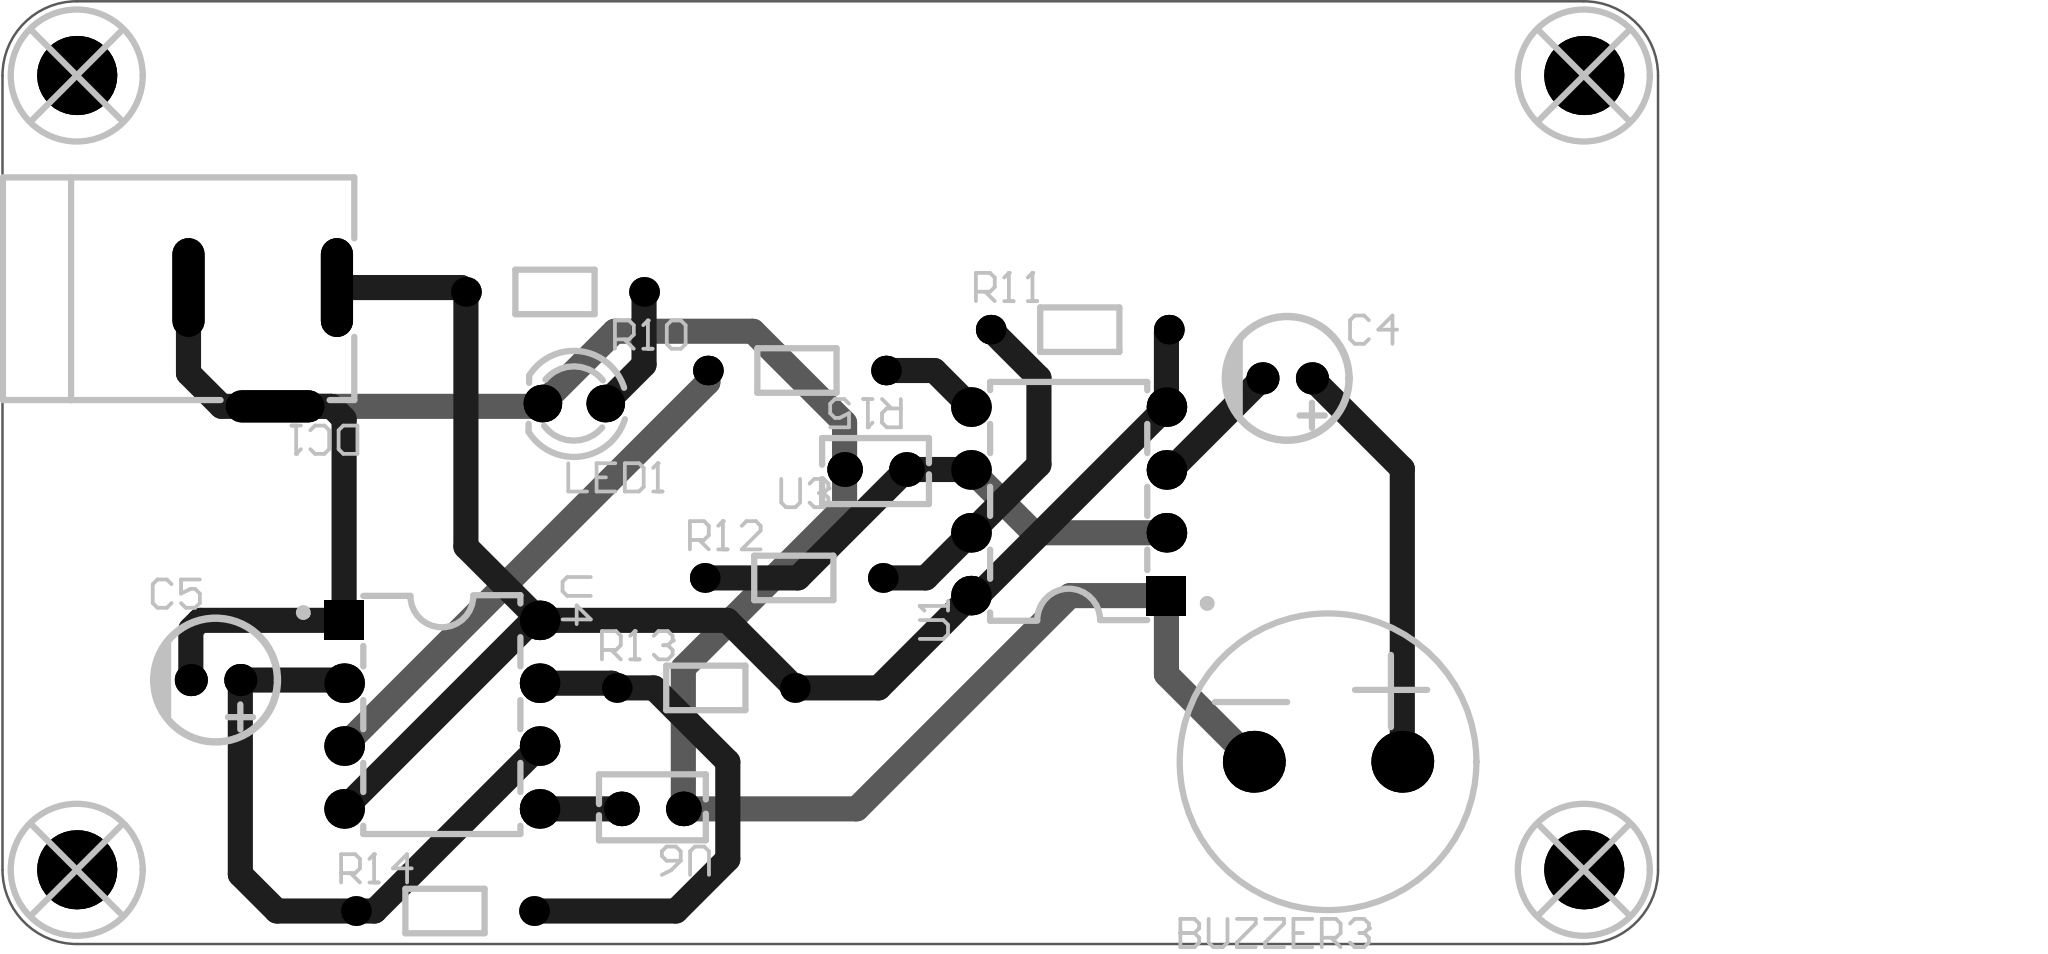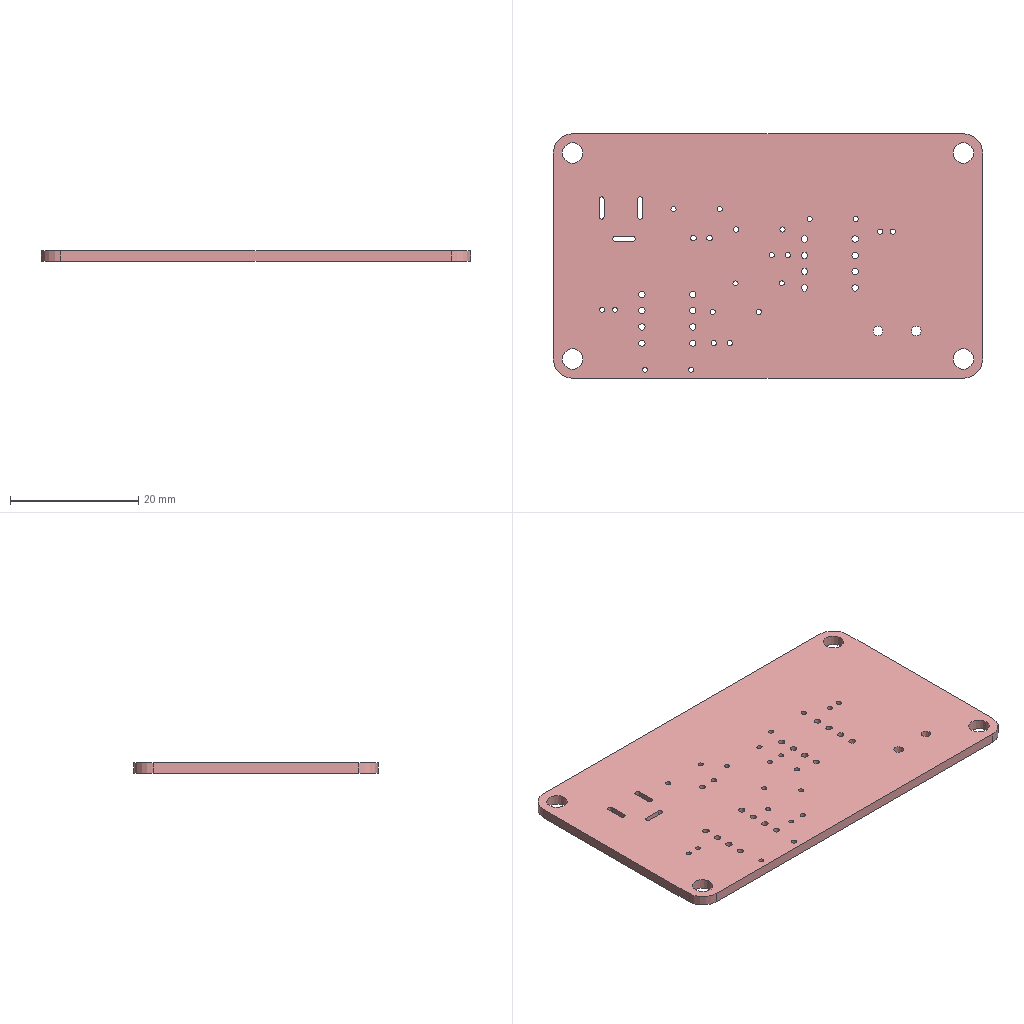Circuit board layout | Altium Designer | box 66.9 x 38.1 x 1.6 mm
Layer stack:
# Altium Designer layer stack of  (unit mm; dielectric type: 0 none, 1 core, 2 prepreg, 3 surface material)
index,name,kind,layer,copper_thickness_mm,dielectric_type,dielectric_thickness_mm,dielectric_material,dielectric_constant
0,Top Paste Mask Layer,other,,,,,,
1,Top Silkscreen Layer,other,,,,,,
2,Top Solder Mask Layer,dielectric,,,3,0.01,,3.3
3,Top Layer,copper,Top Layer,0.035,,,,
4,Dielectric1,dielectric,,,3,1.51,FR4,4.5
5,Bottom Layer,copper,Bottom Layer,0.035,,,,
6,Bottom Solder Mask Layer,dielectric,,,3,0.01,,3.3
7,Bottom Silkscreen Layer,other,,,,,,
8,Bottom Paste Mask Layer,other,,,,,,
# drill layer pairs: low layer,high layer
drill_pair,Top Layer,Bottom Layer
Part placement:
Designator,Comment,Layer,Footprint,Center-X(mm),Center-Y(mm),Rotation
C4,10uF,TopLayer,CAP-TH_BD5.0-P2.00-D0.8-FD,128.143,99.06,180
C5,47uF,TopLayer,CAP-TH_BD5.0-P2.00-D0.8-FD,84.836,86.868,180
R12,6.8kΩ,TopLayer,Res_1/8W,108.204,90.995,0
R13,1kΩ,TopLayer,Res_1/8W,104.648,86.55,0
R14,15kΩ,TopLayer,Res_1/8W,94.107,77.533,0
R15,5.1kΩ,TopLayer,Res_1/8W,108.331,99.378,180
U4,NE555,TopLayer,PDIP-8_L9.6-W6.4-P2.54-LS7.9-BL-1,93.98,85.471,270
U6,10nF,TopLayer,CAP-TH_L4.0-W2.5-P2.50-D0.5,102.489,81.661,180
SCREW1,,TopLayer,M3螺丝,79.225,79.2,0
SCREW2,,TopLayer,M3螺丝,140.129,79.2,0
SCREW3,,TopLayer,M3螺丝,79.225,111.3,0
SCREW4,,TopLayer,M3螺丝,140.129,111.3,0
U1,NE555,TopLayer,PDIP-8_L9.6-W6.4-P2.54-LS7.9-BL-1,119.312,94.09,90
LED1,,TopLayer,LED_TH-3mm,99.314,98.044,180
R10,1kΩ,TopLayer,Res_1/8W,98.552,102.553,180
R11,4.7kΩ,TopLayer,Res_1/8W,119.761,101.028,0
BUZZER3,buzzer,TopLayer,BUZ-TH_BD12.0-P6.00-D0.9-RD,129.794,83.566,0
U3,100nF,TopLayer,CAP-TH_L4.0-W2.5-P2.50-D0.5,111.506,95.377,0
DC1,,TopLayer,DC-2.0,86.741,100.33,180
Pad and via stacks:
# Altium Designer via and pad stacks of  (unit mm). Each distinct definition once, with the count of objects using it.
# via: kind,start_layer,end_layer,hole_mm,diameter_mm,mode(0 simple;1 top-mid-bottom;2 full stack),diameter_per_layer,count,example_net
# pad: kind,layer,hole_mm,hole_type(0 round;1 square;2 slot),plating,top_size,top_shape(1 round;2 rect;3 octagon;9 rounded rect),mid_size,bottom_size,mode,footprint,size_per_layer,count,example
pad,Multi-Layer,0.8,0,plated,1.3x1.3,1,1.3x1.3,1.3x1.3,0,CAP-TH_BD5.0-P2.00-D0.8-FD,,4,C4.1
pad,Multi-Layer,0.8001,0,plated,1.199x1.199,1,1.199x1.199,1.199x1.199,0,Res_1/8W,,12,R12.1
pad,Multi-Layer,1,0,plated,1.6x1.6,1,1.6x1.6,1.6x1.6,0,PDIP-8_L9.6-W6.4-P2.54-LS7.9-BL-1,,14,U4.8
pad,Multi-Layer,1,0,plated,1.6x1.6,2,1.6x1.6,1.6x1.6,0,PDIP-8_L9.6-W6.4-P2.54-LS7.9-BL-1,,2,U4.1
pad,Multi-Layer,0.8,0,plated,1.4x1.4,1,1.4x1.4,1.4x1.4,0,CAP-TH_L4.0-W2.5-P2.50-D0.5,,4,U6.2
pad,Multi-Layer,3.2,0,plated,3.2x3.2,1,3.2x3.2,3.2x3.2,0,M3\u00C2\u00DD\u00CB\u00BF,,4,SCREW1.1
pad,Multi-Layer,0.9144,0,plated,1.524x1.524,1,1.524x1.524,1.524x1.524,0,LED_TH-3mm,,2,LED1.1
pad,Multi-Layer,1.5,0,plated,2.5x2.5,1,2.5x2.5,2.5x2.5,0,BUZ-TH_BD12.0-P6.00-D0.9-RD,,2,BUZZER3.1
pad,Multi-Layer,0.8001,2,plated,4x1.3,1,4x1.3,4x1.3,0,DC-2.0,,3,DC1.2